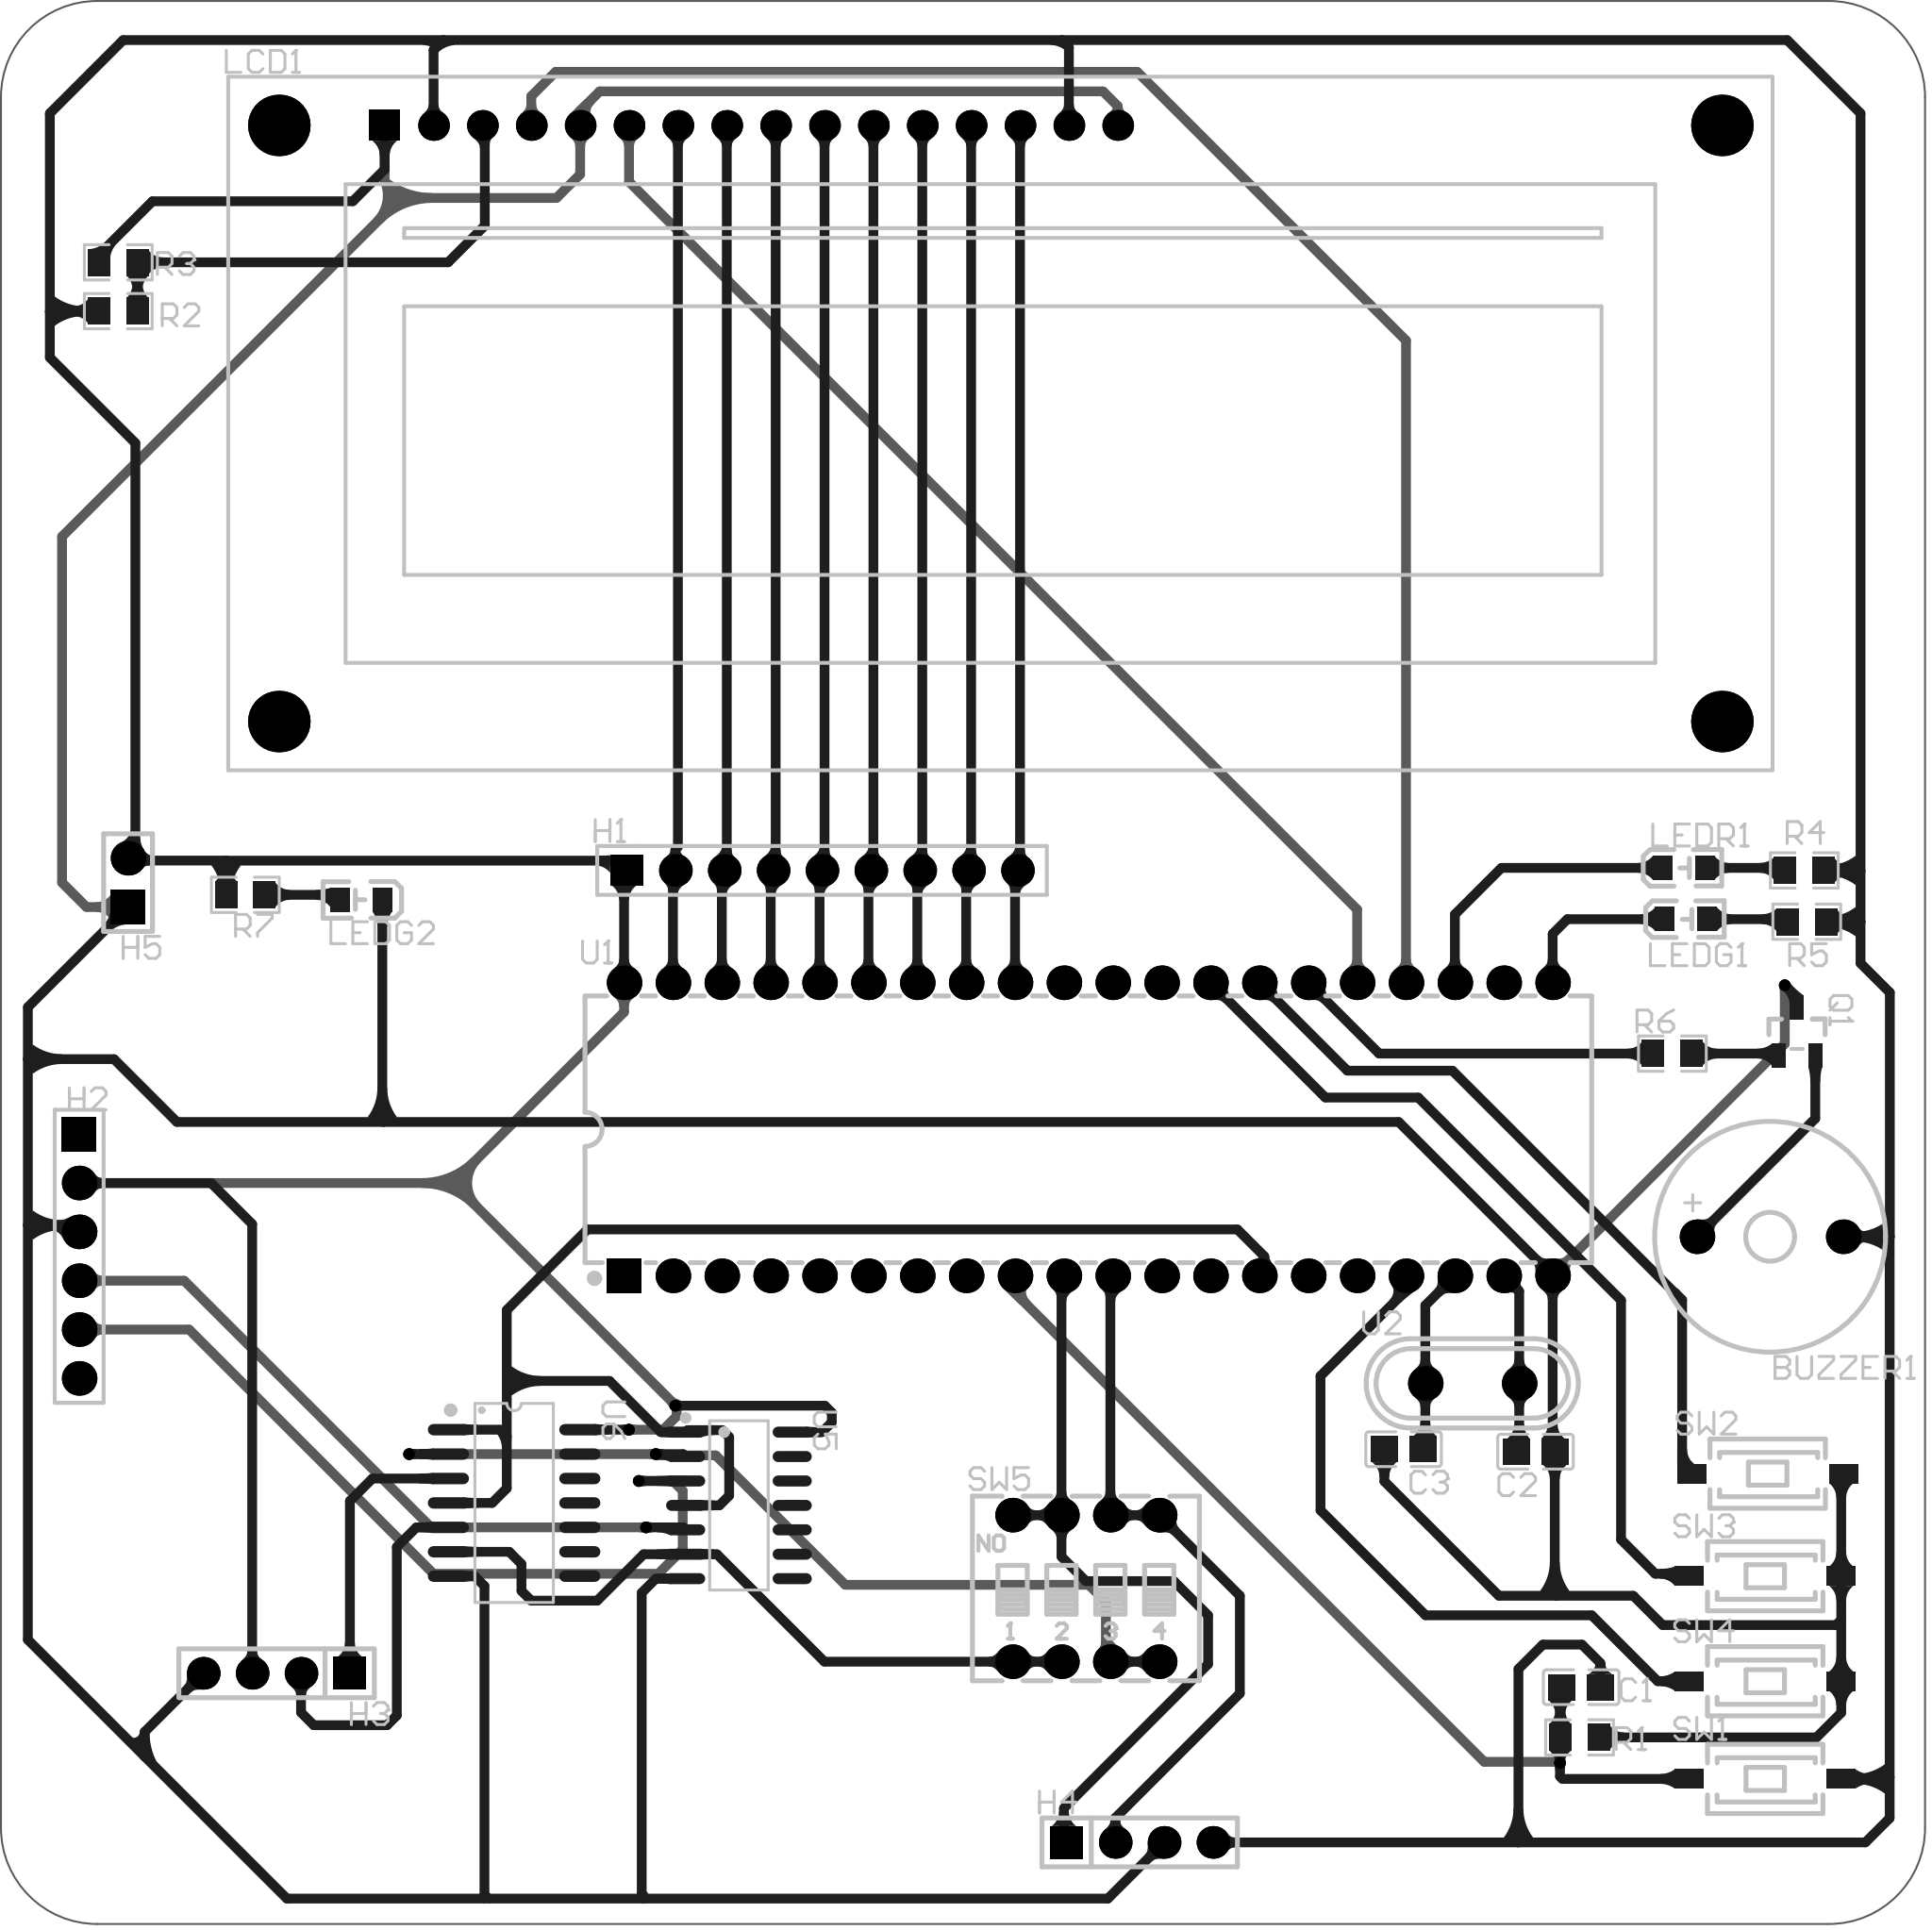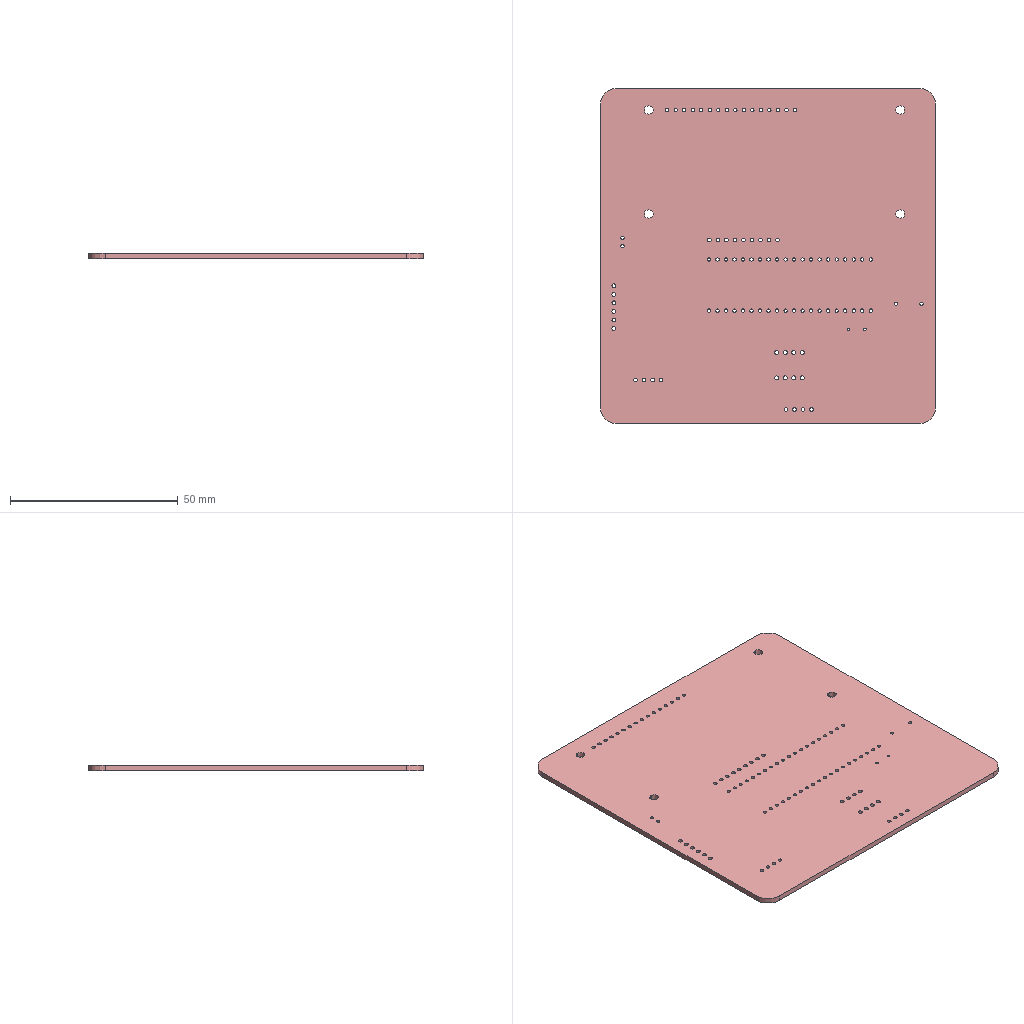Circuit board layout | Altium Designer | box 100 x 100 x 1.6 mm
Layer stack:
# Altium Designer layer stack of  (unit mm; dielectric type: 0 none, 1 core, 2 prepreg, 3 surface material)
index,name,kind,layer,copper_thickness_mm,dielectric_type,dielectric_thickness_mm,dielectric_material,dielectric_constant
0,Top Paste Mask Layer,other,,,,,,
1,Top Silkscreen Layer,other,,,,,,
2,Top Solder Mask Layer,dielectric,,,3,0.01,,3.3
3,Top Layer,copper,Top Layer,0.035,,,,
4,Dielectric1,dielectric,,,3,1.51,FR4,4.5
5,Bottom Layer,copper,Bottom Layer,0.035,,,,
6,Bottom Solder Mask Layer,dielectric,,,3,0.01,,3.3
7,Bottom Silkscreen Layer,other,,,,,,
8,Bottom Paste Mask Layer,other,,,,,,
# drill layer pairs: low layer,high layer
drill_pair,Top Layer,Bottom Layer
Part placement:
Designator,Comment,Layer,Footprint,Center-X(mm),Center-Y(mm),Rotation
BUZZER1,buzzer-12X9,TopLayer,BUZ-TH_BD12.0-P7.60-D0.6-FD,168.148,111.938,0
C1,10uf,TopLayer,C0805,158.327,88.516,0
C2,30pf,TopLayer,C0805,149.098,100.889,0
C3,30pf,TopLayer,C0805,155.956,100.762,180
H1,,TopLayer,HDR-TH_9P-P2.54-V-F-1,118.872,130.988,0
H2,,TopLayer,HDR-TH_6P-P2.54-V-M-1,80.264,110.922,270
H3,,TopLayer,HDR-TH_4P-P2.54-V-M,90.526,89.239,180
H4,,TopLayer,HDR-TH_4P-P2.54-V-M,135.382,80.442,0
LCD1,LMB162ADC,TopLayer,LCD1602,128.143,154.229,0
LEDG1,,TopLayer,LED_0805,163.78,128.453,0
LEDR1,,TopLayer,LED_0805,163.653,131.12,0
Q1,2N3906S-RTK/PS,TopLayer,SOT-23-3_L2.9-W1.3-P1.90-LS2.4-TR,169.545,122.606,270
R1,10K,TopLayer,R0805,158.242,85.903,0
R2,10K,TopLayer,R0805,82.296,160.071,180
R3,1K,TopLayer,R0805,82.296,162.611,0
R4,220,TopLayer,R0805,169.926,130.988,0
R5,220,TopLayer,R0805,170.053,128.321,0
R6,2.2K,TopLayer,R0805,163.068,121.463,0
SW5,DSWB04LHGET,TopLayer,SW-TH_DSWB04LHGET,132.588,93.65,0
U1,STC89C516RD+40I-PDIP40,TopLayer,DIP-40_L52.3-W13.9-P2.54-LS15.2-BL,132.715,117.526,0
U2,11.059MHz,TopLayer,HC-49US_L11.0-W4.6-P4.88,152.667,104.313,0
U5,SN74LS126ADR2,TopLayer,SOIC-14_L8.7-W3.9-P1.27-LS6.0-BL,114.554,97.968,270
U6,DM74LS125ASJ,TopLayer,SOP-14_L10.2-W5.3-P1.27-LS7.8-BL,102.87,98.095,270
LEDG2,,TopLayer,LED_0805,94.919,129.459,180
R7,220,TopLayer,R0805,88.9,129.718,180
H5,,TopLayer,HDR-TH_2P-P2.54-V-M-1,82.804,130.353,90
SW1,Tact switch 3*6*2.5,TopLayer,SW-SMD_L6.0-W3.6-LS8.0,167.894,83.744,0
SW2,Tact switch 3*6*2.5,TopLayer,SW-SMD_L6.0-W3.6-LS8.0,168.021,99.619,0
SW3,Tact switch 3*6*2.5,TopLayer,SW-SMD_L6.0-W3.6-LS8.0,167.894,94.285,0
SW4,Tact switch 3*6*2.5,TopLayer,SW-SMD_L6.0-W3.6-LS8.0,167.894,88.824,0
Pad and via stacks:
# Altium Designer via and pad stacks of  (unit mm). Each distinct definition once, with the count of objects using it.
# via: kind,start_layer,end_layer,hole_mm,diameter_mm,mode(0 simple;1 top-mid-bottom;2 full stack),diameter_per_layer,count,example_net
# pad: kind,layer,hole_mm,hole_type(0 round;1 square;2 slot),plating,top_size,top_shape(1 round;2 rect;3 octagon;9 rounded rect),mid_size,bottom_size,mode,footprint,size_per_layer,count,example
pad,Multi-Layer,1,0,plated,1.8x1.8,1,1.8x1.8,1.8x1.8,0,BUZ-TH_BD12.0-P7.60-D0.6-FD,,2,BUZZER1.2
pad,Multi-Layer,1.1,0,plated,1.7x1.575,2,1.7x1.575,1.7x1.575,0,HDR-TH_9P-P2.54-V-F-1,,1,H1.1
pad,Multi-Layer,1.1,0,plated,1.7x1.7,1,1.7x1.7,1.7x1.7,0,HDR-TH_9P-P2.54-V-F-1,,8,H1.2
pad,Multi-Layer,1.2,0,plated,1.8x1.8,1,1.8x1.8,1.8x1.8,0,HDR-TH_6P-P2.54-V-M-1,,5,H2.6
pad,Multi-Layer,1.2,0,plated,1.8x1.8,2,1.8x1.8,1.8x1.8,0,HDR-TH_6P-P2.54-V-M-1,,1,H2.1
pad,Multi-Layer,1.1,0,plated,1.7x1.7,2,1.7x1.7,1.7x1.7,0,HDR-TH_4P-P2.54-V-M,,2,H3.1
pad,Multi-Layer,1.1,0,plated,1.7x1.7,1,1.7x1.7,1.7x1.7,0,HDR-TH_4P-P2.54-V-M,,6,H3.2
pad,Multi-Layer,1,0,plated,1.6x1.6,1,1.6x1.6,1.6x1.6,0,LCD1602,,15,LCD1.16
pad,Multi-Layer,1,0,plated,1.6x1.6,2,1.6x1.6,1.6x1.6,0,LCD1602,,1,LCD1.1
pad,Multi-Layer,2.5,2,plated,3.2x3.2,1,3.2x3.2,3.2x3.2,0,LCD1602,,4,LCD1.0
pad,Multi-Layer,1.2,0,plated,1.8x1.8,1,1.8x1.8,1.8x1.8,0,SW-TH_DSWB04LHGET,,8,SW5.5
pad,Multi-Layer,1,0,plated,1.8x1.8,1,1.8x1.8,1.8x1.8,0,DIP-40_L52.3-W13.9-P2.54-LS15.2-BL,,39,U1.19
pad,Multi-Layer,1,0,plated,1.8x1.8,2,1.8x1.8,1.8x1.8,0,DIP-40_L52.3-W13.9-P2.54-LS15.2-BL,,1,U1.1
pad,Multi-Layer,0.8,0,plated,1.8x1.8,1,1.8x1.8,1.8x1.8,0,HC-49US_L11.0-W4.6-P4.88,,2,U2.1
pad,Multi-Layer,1,0,plated,1.8x1.8,1,1.8x1.8,1.8x1.8,0,HDR-TH_2P-P2.54-V-M-1,,1,H5.2
pad,Multi-Layer,1,0,plated,1.8x1.8,2,1.8x1.8,1.8x1.8,0,HDR-TH_2P-P2.54-V-M-1,,1,H5.1
pad,Top Layer,0,0,plated,1.41x1.35,2,1.41x1.35,1.41x1.35,0,C0805,,6,C1.2
pad,Top Layer,0,0,plated,1x1.25,2,1x1.25,1x1.25,0,LED_0805,,6,LEDG1.2
pad,Top Layer,0,0,plated,0.7x1.25,2,0.7x1.25,0.7x1.25,0,SOT-23-3_L2.9-W1.3-P1.90-LS2.4-TR,,3,Q1.3
pad,Top Layer,0,0,plated,1.133x1.377,2,1.133x1.377,1.133x1.377,0,R0805,,14,R1.2
pad,Top Layer,0,0,plated,0.574x2.038,1,0.574x2.038,0.574x2.038,0,SOIC-14_L8.7-W3.9-P1.27-LS6.0-BL,,14,U5.1
pad,Top Layer,0,0,plated,0.595x2.143,1,0.595x2.143,0.595x2.143,0,SOP-14_L10.2-W5.3-P1.27-LS7.8-BL,,14,U6.1
pad,Top Layer,0,0,plated,1.5x1,2,1.5x1,1.5x1,0,SW-SMD_L6.0-W3.6-LS8.0,,8,SW1.1
via,Top Layer,Bottom Layer,0.3048,0.6096,0,,7,RX1
via,Top Layer,Bottom Layer,0.3048,0.61,0,,1,$1N2914